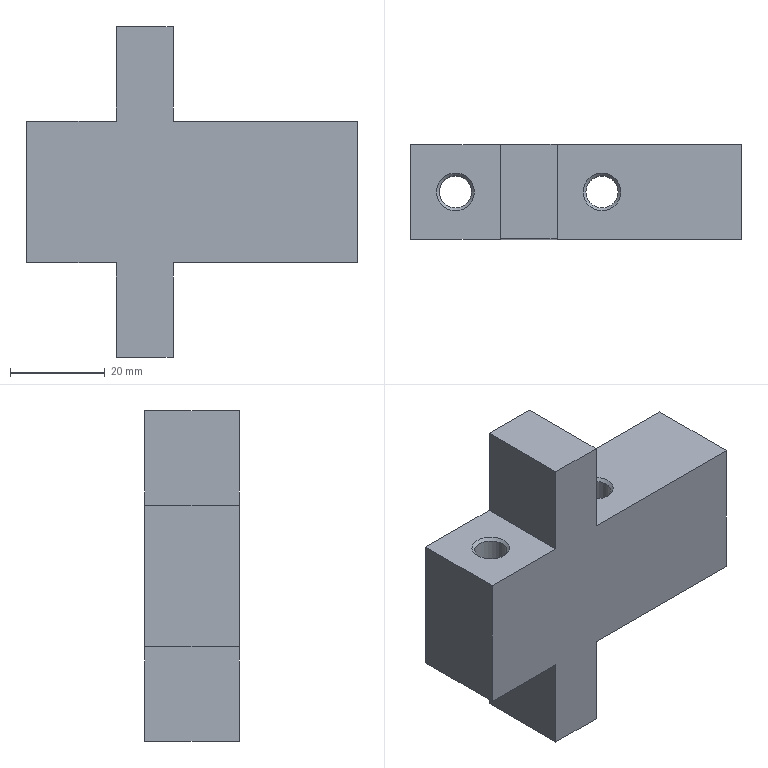Part | STEP file | 冲床-300配套压波_id182_x_t | 1 solid | 20 faces | box 70 x 20 x 70 mm | volume 49405 mm3 | plane 14 | cone 4 | cylinder 2 | commonest cylinder face diameters 6.8 x2
STEP:
#1=CARTESIAN_POINT('',(1118.5,-185.,50.));
#2=VERTEX_POINT('',#1);
#3=CARTESIAN_POINT('',(1114.5,-185.,50.));
#4=DIRECTION('',(0.,0.,-1.));
#5=DIRECTION('',(1.,0.,0.));
#6=AXIS2_PLACEMENT_3D('',#3,#4,#5);
#7=CIRCLE('',#6,4.);
#8=EDGE_CURVE('',#2,#2,#7,.T.);
#9=ORIENTED_EDGE('',*,*,#8,.T.);
#10=EDGE_LOOP('',(#9));
#11=FACE_BOUND('',#10,.T.);
#12=CARTESIAN_POINT('',(1105.,-175.,50.));
#13=VERTEX_POINT('',#12);
#14=CARTESIAN_POINT('',(1124.,-175.,50.));
#15=VERTEX_POINT('',#14);
#16=CARTESIAN_POINT('',(1155.,-175.,50.));
#17=DIRECTION('',(1.,0.,0.));
#18=VECTOR('',#17,1.);
#19=LINE('',#16,#18);
#20=EDGE_CURVE('',#13,#15,#19,.T.);
#21=ORIENTED_EDGE('',*,*,#20,.F.);
#22=CARTESIAN_POINT('',(1105.,-195.,50.));
#23=VERTEX_POINT('',#22);
#24=CARTESIAN_POINT('',(1105.,-175.,50.));
#25=DIRECTION('',(0.,1.,0.));
#26=VECTOR('',#25,1.);
#27=LINE('',#24,#26);
#28=EDGE_CURVE('',#23,#13,#27,.T.);
#29=ORIENTED_EDGE('',*,*,#28,.F.);
#30=CARTESIAN_POINT('',(1124.,-195.,50.));
#31=VERTEX_POINT('',#30);
#32=CARTESIAN_POINT('',(1155.,-195.,50.));
#33=DIRECTION('',(1.,0.,0.));
#34=VECTOR('',#33,1.);
#35=LINE('',#32,#34);
#36=EDGE_CURVE('',#23,#31,#35,.T.);
#37=ORIENTED_EDGE('',*,*,#36,.T.);
#38=CARTESIAN_POINT('',(1124.,-175.,50.));
#39=DIRECTION('',(0.,1.,0.));
#40=VECTOR('',#39,1.);
#41=LINE('',#38,#40);
#42=EDGE_CURVE('',#31,#15,#41,.T.);
#43=ORIENTED_EDGE('',*,*,#42,.T.);
#44=EDGE_LOOP('',(#21,#29,#37,#43));
#45=FACE_BOUND('',#44,.T.);
#46=CARTESIAN_POINT('',(1155.,-175.,50.));
#47=DIRECTION('',(0.,0.,1.));
#48=DIRECTION('',(-1.,0.,0.));
#49=AXIS2_PLACEMENT_3D('',#46,#47,#48);
#50=PLANE('',#49);
#51=ADVANCED_FACE('',(#11,#45),#50,.T.);
#52=CARTESIAN_POINT('',(1124.,-195.,70.));
#53=VERTEX_POINT('',#52);
#54=CARTESIAN_POINT('',(1124.,-195.,50.));
#55=DIRECTION('',(0.,0.,-1.));
#56=VECTOR('',#55,1.);
#57=LINE('',#54,#56);
#58=EDGE_CURVE('',#53,#31,#57,.T.);
#59=ORIENTED_EDGE('',*,*,#58,.F.);
#60=CARTESIAN_POINT('',(1124.,-175.,70.));
#61=VERTEX_POINT('',#60);
#62=CARTESIAN_POINT('',(1124.,-175.,70.));
#63=DIRECTION('',(0.,1.,0.));
#64=VECTOR('',#63,1.);
#65=LINE('',#62,#64);
#66=EDGE_CURVE('',#53,#61,#65,.T.);
#67=ORIENTED_EDGE('',*,*,#66,.T.);
#68=CARTESIAN_POINT('',(1124.,-175.,50.));
#69=DIRECTION('',(0.,0.,-1.));
#70=VECTOR('',#69,1.);
#71=LINE('',#68,#70);
#72=EDGE_CURVE('',#61,#15,#71,.T.);
#73=ORIENTED_EDGE('',*,*,#72,.T.);
#74=ORIENTED_EDGE('',*,*,#42,.F.);
#75=EDGE_LOOP('',(#59,#67,#73,#74));
#76=FACE_OUTER_BOUND('',#75,.T.);
#77=CARTESIAN_POINT('',(1124.,-175.,50.));
#78=DIRECTION('',(-1.,0.,0.));
#79=DIRECTION('',(0.,0.,1.));
#80=AXIS2_PLACEMENT_3D('',#77,#78,#79);
#81=PLANE('',#80);
#82=ADVANCED_FACE('',(#76),#81,.T.);
#83=CARTESIAN_POINT('',(1136.,-195.,70.));
#84=VERTEX_POINT('',#83);
#85=CARTESIAN_POINT('',(1124.,-195.,70.));
#86=DIRECTION('',(-1.,0.,0.));
#87=VECTOR('',#86,1.);
#88=LINE('',#85,#87);
#89=EDGE_CURVE('',#84,#53,#88,.T.);
#90=ORIENTED_EDGE('',*,*,#89,.F.);
#91=CARTESIAN_POINT('',(1136.,-175.,70.));
#92=VERTEX_POINT('',#91);
#93=CARTESIAN_POINT('',(1136.,-175.,70.));
#94=DIRECTION('',(0.,1.,0.));
#95=VECTOR('',#94,1.);
#96=LINE('',#93,#95);
#97=EDGE_CURVE('',#84,#92,#96,.T.);
#98=ORIENTED_EDGE('',*,*,#97,.T.);
#99=CARTESIAN_POINT('',(1124.,-175.,70.));
#100=DIRECTION('',(-1.,0.,0.));
#101=VECTOR('',#100,1.);
#102=LINE('',#99,#101);
#103=EDGE_CURVE('',#92,#61,#102,.T.);
#104=ORIENTED_EDGE('',*,*,#103,.T.);
#105=ORIENTED_EDGE('',*,*,#66,.F.);
#106=EDGE_LOOP('',(#90,#98,#104,#105));
#107=FACE_OUTER_BOUND('',#106,.T.);
#108=CARTESIAN_POINT('',(1124.,-175.,70.));
#109=DIRECTION('',(0.,0.,1.));
#110=DIRECTION('',(1.,0.,0.));
#111=AXIS2_PLACEMENT_3D('',#108,#109,#110);
#112=PLANE('',#111);
#113=ADVANCED_FACE('',(#107),#112,.T.);
#114=CARTESIAN_POINT('',(1136.,-195.,50.));
#115=VERTEX_POINT('',#114);
#116=CARTESIAN_POINT('',(1136.,-195.,70.));
#117=DIRECTION('',(0.,0.,1.));
#118=VECTOR('',#117,1.);
#119=LINE('',#116,#118);
#120=EDGE_CURVE('',#115,#84,#119,.T.);
#121=ORIENTED_EDGE('',*,*,#120,.F.);
#122=CARTESIAN_POINT('',(1136.,-175.,50.));
#123=VERTEX_POINT('',#122);
#124=CARTESIAN_POINT('',(1136.,-175.,50.));
#125=DIRECTION('',(0.,1.,0.));
#126=VECTOR('',#125,1.);
#127=LINE('',#124,#126);
#128=EDGE_CURVE('',#115,#123,#127,.T.);
#129=ORIENTED_EDGE('',*,*,#128,.T.);
#130=CARTESIAN_POINT('',(1136.,-175.,70.));
#131=DIRECTION('',(0.,0.,1.));
#132=VECTOR('',#131,1.);
#133=LINE('',#130,#132);
#134=EDGE_CURVE('',#123,#92,#133,.T.);
#135=ORIENTED_EDGE('',*,*,#134,.T.);
#136=ORIENTED_EDGE('',*,*,#97,.F.);
#137=EDGE_LOOP('',(#121,#129,#135,#136));
#138=FACE_OUTER_BOUND('',#137,.T.);
#139=CARTESIAN_POINT('',(1136.,-175.,70.));
#140=DIRECTION('',(1.,0.,0.));
#141=DIRECTION('',(0.,0.,-1.));
#142=AXIS2_PLACEMENT_3D('',#139,#140,#141);
#143=PLANE('',#142);
#144=ADVANCED_FACE('',(#138),#143,.T.);
#145=CARTESIAN_POINT('',(1149.5,-185.,50.));
#146=VERTEX_POINT('',#145);
#147=CARTESIAN_POINT('',(1145.5,-185.,50.));
#148=DIRECTION('',(0.,0.,-1.));
#149=DIRECTION('',(1.,0.,0.));
#150=AXIS2_PLACEMENT_3D('',#147,#148,#149);
#151=CIRCLE('',#150,4.);
#152=EDGE_CURVE('',#146,#146,#151,.T.);
#153=ORIENTED_EDGE('',*,*,#152,.T.);
#154=EDGE_LOOP('',(#153));
#155=FACE_BOUND('',#154,.T.);
#156=ORIENTED_EDGE('',*,*,#128,.F.);
#157=CARTESIAN_POINT('',(1175.,-195.,50.));
#158=VERTEX_POINT('',#157);
#159=CARTESIAN_POINT('',(1155.,-195.,50.));
#160=DIRECTION('',(1.,0.,0.));
#161=VECTOR('',#160,1.);
#162=LINE('',#159,#161);
#163=EDGE_CURVE('',#115,#158,#162,.T.);
#164=ORIENTED_EDGE('',*,*,#163,.T.);
#165=CARTESIAN_POINT('',(1175.,-175.,50.));
#166=VERTEX_POINT('',#165);
#167=CARTESIAN_POINT('',(1175.,-175.,50.));
#168=DIRECTION('',(0.,1.,0.));
#169=VECTOR('',#168,1.);
#170=LINE('',#167,#169);
#171=EDGE_CURVE('',#158,#166,#170,.T.);
#172=ORIENTED_EDGE('',*,*,#171,.T.);
#173=CARTESIAN_POINT('',(1155.,-175.,50.));
#174=DIRECTION('',(1.,0.,0.));
#175=VECTOR('',#174,1.);
#176=LINE('',#173,#175);
#177=EDGE_CURVE('',#123,#166,#176,.T.);
#178=ORIENTED_EDGE('',*,*,#177,.F.);
#179=EDGE_LOOP('',(#156,#164,#172,#178));
#180=FACE_BOUND('',#179,.T.);
#181=CARTESIAN_POINT('',(1155.,-175.,50.));
#182=DIRECTION('',(0.,0.,1.));
#183=DIRECTION('',(-1.,0.,0.));
#184=AXIS2_PLACEMENT_3D('',#181,#182,#183);
#185=PLANE('',#184);
#186=ADVANCED_FACE('',(#155,#180),#185,.T.);
#187=CARTESIAN_POINT('',(1175.,-175.,20.));
#188=VERTEX_POINT('',#187);
#189=CARTESIAN_POINT('',(1175.,-175.,50.));
#190=DIRECTION('',(0.,0.,1.));
#191=VECTOR('',#190,1.);
#192=LINE('',#189,#191);
#193=EDGE_CURVE('',#188,#166,#192,.T.);
#194=ORIENTED_EDGE('',*,*,#193,.T.);
#195=ORIENTED_EDGE('',*,*,#171,.F.);
#196=CARTESIAN_POINT('',(1175.,-195.,20.));
#197=VERTEX_POINT('',#196);
#198=CARTESIAN_POINT('',(1175.,-195.,50.));
#199=DIRECTION('',(0.,0.,1.));
#200=VECTOR('',#199,1.);
#201=LINE('',#198,#200);
#202=EDGE_CURVE('',#197,#158,#201,.T.);
#203=ORIENTED_EDGE('',*,*,#202,.F.);
#204=CARTESIAN_POINT('',(1175.,-175.,20.));
#205=DIRECTION('',(0.,1.,0.));
#206=VECTOR('',#205,1.);
#207=LINE('',#204,#206);
#208=EDGE_CURVE('',#197,#188,#207,.T.);
#209=ORIENTED_EDGE('',*,*,#208,.T.);
#210=EDGE_LOOP('',(#194,#195,#203,#209));
#211=FACE_OUTER_BOUND('',#210,.T.);
#212=CARTESIAN_POINT('',(1175.,-175.,50.));
#213=DIRECTION('',(-1.,0.,0.));
#214=DIRECTION('',(0.,0.,-1.));
#215=AXIS2_PLACEMENT_3D('',#212,#213,#214);
#216=PLANE('',#215);
#217=ADVANCED_FACE('',(#211),#216,.F.);
#218=CARTESIAN_POINT('',(1141.5,-185.,20.));
#219=VERTEX_POINT('',#218);
#220=CARTESIAN_POINT('',(1145.5,-185.,20.));
#221=DIRECTION('',(0.,0.,1.));
#222=DIRECTION('',(-1.,0.,0.));
#223=AXIS2_PLACEMENT_3D('',#220,#221,#222);
#224=CIRCLE('',#223,4.);
#225=EDGE_CURVE('',#219,#219,#224,.T.);
#226=ORIENTED_EDGE('',*,*,#225,.T.);
#227=EDGE_LOOP('',(#226));
#228=FACE_BOUND('',#227,.T.);
#229=CARTESIAN_POINT('',(1136.,-175.,20.));
#230=VERTEX_POINT('',#229);
#231=CARTESIAN_POINT('',(1155.,-175.,20.));
#232=DIRECTION('',(-1.,0.,0.));
#233=VECTOR('',#232,1.);
#234=LINE('',#231,#233);
#235=EDGE_CURVE('',#188,#230,#234,.T.);
#236=ORIENTED_EDGE('',*,*,#235,.F.);
#237=ORIENTED_EDGE('',*,*,#208,.F.);
#238=CARTESIAN_POINT('',(1136.,-195.,20.));
#239=VERTEX_POINT('',#238);
#240=CARTESIAN_POINT('',(1155.,-195.,20.));
#241=DIRECTION('',(-1.,0.,0.));
#242=VECTOR('',#241,1.);
#243=LINE('',#240,#242);
#244=EDGE_CURVE('',#197,#239,#243,.T.);
#245=ORIENTED_EDGE('',*,*,#244,.T.);
#246=CARTESIAN_POINT('',(1136.,-175.,20.));
#247=DIRECTION('',(0.,1.,0.));
#248=VECTOR('',#247,1.);
#249=LINE('',#246,#248);
#250=EDGE_CURVE('',#239,#230,#249,.T.);
#251=ORIENTED_EDGE('',*,*,#250,.T.);
#252=EDGE_LOOP('',(#236,#237,#245,#251));
#253=FACE_BOUND('',#252,.T.);
#254=CARTESIAN_POINT('',(1155.,-185.,20.));
#255=DIRECTION('',(0.,0.,-1.));
#256=DIRECTION('',(-1.,0.,0.));
#257=AXIS2_PLACEMENT_3D('',#254,#255,#256);
#258=PLANE('',#257);
#259=ADVANCED_FACE('',(#228,#253),#258,.T.);
#260=CARTESIAN_POINT('',(1110.5,-185.,20.));
#261=VERTEX_POINT('',#260);
#262=CARTESIAN_POINT('',(1114.5,-185.,20.));
#263=DIRECTION('',(0.,0.,1.));
#264=DIRECTION('',(-1.,0.,0.));
#265=AXIS2_PLACEMENT_3D('',#262,#263,#264);
#266=CIRCLE('',#265,4.);
#267=EDGE_CURVE('',#261,#261,#266,.T.);
#268=ORIENTED_EDGE('',*,*,#267,.T.);
#269=EDGE_LOOP('',(#268));
#270=FACE_BOUND('',#269,.T.);
#271=CARTESIAN_POINT('',(1124.,-195.,20.));
#272=VERTEX_POINT('',#271);
#273=CARTESIAN_POINT('',(1105.,-195.,20.));
#274=VERTEX_POINT('',#273);
#275=CARTESIAN_POINT('',(1155.,-195.,20.));
#276=DIRECTION('',(-1.,0.,0.));
#277=VECTOR('',#276,1.);
#278=LINE('',#275,#277);
#279=EDGE_CURVE('',#272,#274,#278,.T.);
#280=ORIENTED_EDGE('',*,*,#279,.T.);
#281=CARTESIAN_POINT('',(1105.,-175.,20.));
#282=VERTEX_POINT('',#281);
#283=CARTESIAN_POINT('',(1105.,-175.,20.));
#284=DIRECTION('',(0.,-1.,0.));
#285=VECTOR('',#284,1.);
#286=LINE('',#283,#285);
#287=EDGE_CURVE('',#282,#274,#286,.T.);
#288=ORIENTED_EDGE('',*,*,#287,.F.);
#289=CARTESIAN_POINT('',(1124.,-175.,20.));
#290=VERTEX_POINT('',#289);
#291=CARTESIAN_POINT('',(1155.,-175.,20.));
#292=DIRECTION('',(-1.,0.,0.));
#293=VECTOR('',#292,1.);
#294=LINE('',#291,#293);
#295=EDGE_CURVE('',#290,#282,#294,.T.);
#296=ORIENTED_EDGE('',*,*,#295,.F.);
#297=CARTESIAN_POINT('',(1124.,-175.,20.));
#298=DIRECTION('',(0.,-1.,0.));
#299=VECTOR('',#298,1.);
#300=LINE('',#297,#299);
#301=EDGE_CURVE('',#290,#272,#300,.T.);
#302=ORIENTED_EDGE('',*,*,#301,.T.);
#303=EDGE_LOOP('',(#280,#288,#296,#302));
#304=FACE_BOUND('',#303,.T.);
#305=CARTESIAN_POINT('',(1155.,-185.,20.));
#306=DIRECTION('',(0.,0.,-1.));
#307=DIRECTION('',(-1.,0.,0.));
#308=AXIS2_PLACEMENT_3D('',#305,#306,#307);
#309=PLANE('',#308);
#310=ADVANCED_FACE('',(#270,#304),#309,.T.);
#311=CARTESIAN_POINT('',(1105.,-195.,50.));
#312=DIRECTION('',(0.,0.,1.));
#313=VECTOR('',#312,1.);
#314=LINE('',#311,#313);
#315=EDGE_CURVE('',#274,#23,#314,.T.);
#316=ORIENTED_EDGE('',*,*,#315,.T.);
#317=ORIENTED_EDGE('',*,*,#28,.T.);
#318=CARTESIAN_POINT('',(1105.,-175.,50.));
#319=DIRECTION('',(0.,0.,1.));
#320=VECTOR('',#319,1.);
#321=LINE('',#318,#320);
#322=EDGE_CURVE('',#282,#13,#321,.T.);
#323=ORIENTED_EDGE('',*,*,#322,.F.);
#324=ORIENTED_EDGE('',*,*,#287,.T.);
#325=EDGE_LOOP('',(#316,#317,#323,#324));
#326=FACE_OUTER_BOUND('',#325,.T.);
#327=CARTESIAN_POINT('',(1105.,-175.,50.));
#328=DIRECTION('',(-1.,0.,0.));
#329=DIRECTION('',(0.,0.,-1.));
#330=AXIS2_PLACEMENT_3D('',#327,#328,#329);
#331=PLANE('',#330);
#332=ADVANCED_FACE('',(#326),#331,.T.);
#333=ORIENTED_EDGE('',*,*,#322,.T.);
#334=ORIENTED_EDGE('',*,*,#20,.T.);
#335=ORIENTED_EDGE('',*,*,#72,.F.);
#336=ORIENTED_EDGE('',*,*,#103,.F.);
#337=ORIENTED_EDGE('',*,*,#134,.F.);
#338=ORIENTED_EDGE('',*,*,#177,.T.);
#339=ORIENTED_EDGE('',*,*,#193,.F.);
#340=ORIENTED_EDGE('',*,*,#235,.T.);
#341=CARTESIAN_POINT('',(1136.,-175.,0.));
#342=VERTEX_POINT('',#341);
#343=CARTESIAN_POINT('',(1136.,-175.,0.));
#344=DIRECTION('',(0.,0.,-1.));
#345=VECTOR('',#344,1.);
#346=LINE('',#343,#345);
#347=EDGE_CURVE('',#230,#342,#346,.T.);
#348=ORIENTED_EDGE('',*,*,#347,.T.);
#349=CARTESIAN_POINT('',(1124.,-175.,0.));
#350=VERTEX_POINT('',#349);
#351=CARTESIAN_POINT('',(1124.,-175.,0.));
#352=DIRECTION('',(-1.,0.,0.));
#353=VECTOR('',#352,1.);
#354=LINE('',#351,#353);
#355=EDGE_CURVE('',#342,#350,#354,.T.);
#356=ORIENTED_EDGE('',*,*,#355,.T.);
#357=CARTESIAN_POINT('',(1124.,-175.,20.));
#358=DIRECTION('',(0.,0.,1.));
#359=VECTOR('',#358,1.);
#360=LINE('',#357,#359);
#361=EDGE_CURVE('',#350,#290,#360,.T.);
#362=ORIENTED_EDGE('',*,*,#361,.T.);
#363=ORIENTED_EDGE('',*,*,#295,.T.);
#364=EDGE_LOOP('',(#333,#334,#335,#336,#337,#338,#339,#340,#348,#356,#362,#363));
#365=FACE_OUTER_BOUND('',#364,.T.);
#366=CARTESIAN_POINT('',(1155.,-175.,50.));
#367=DIRECTION('',(0.,1.,0.));
#368=DIRECTION('',(0.,0.,-1.));
#369=AXIS2_PLACEMENT_3D('',#366,#367,#368);
#370=PLANE('',#369);
#371=ADVANCED_FACE('',(#365),#370,.T.);
#372=ORIENTED_EDGE('',*,*,#279,.F.);
#373=CARTESIAN_POINT('',(1124.,-195.,0.));
#374=VERTEX_POINT('',#373);
#375=CARTESIAN_POINT('',(1124.,-195.,20.));
#376=DIRECTION('',(0.,0.,1.));
#377=VECTOR('',#376,1.);
#378=LINE('',#375,#377);
#379=EDGE_CURVE('',#374,#272,#378,.T.);
#380=ORIENTED_EDGE('',*,*,#379,.F.);
#381=CARTESIAN_POINT('',(1136.,-195.,0.));
#382=VERTEX_POINT('',#381);
#383=CARTESIAN_POINT('',(1124.,-195.,0.));
#384=DIRECTION('',(-1.,0.,0.));
#385=VECTOR('',#384,1.);
#386=LINE('',#383,#385);
#387=EDGE_CURVE('',#382,#374,#386,.T.);
#388=ORIENTED_EDGE('',*,*,#387,.F.);
#389=CARTESIAN_POINT('',(1136.,-195.,0.));
#390=DIRECTION('',(0.,0.,-1.));
#391=VECTOR('',#390,1.);
#392=LINE('',#389,#391);
#393=EDGE_CURVE('',#239,#382,#392,.T.);
#394=ORIENTED_EDGE('',*,*,#393,.F.);
#395=ORIENTED_EDGE('',*,*,#244,.F.);
#396=ORIENTED_EDGE('',*,*,#202,.T.);
#397=ORIENTED_EDGE('',*,*,#163,.F.);
#398=ORIENTED_EDGE('',*,*,#120,.T.);
#399=ORIENTED_EDGE('',*,*,#89,.T.);
#400=ORIENTED_EDGE('',*,*,#58,.T.);
#401=ORIENTED_EDGE('',*,*,#36,.F.);
#402=ORIENTED_EDGE('',*,*,#315,.F.);
#403=EDGE_LOOP('',(#372,#380,#388,#394,#395,#396,#397,#398,#399,#400,#401,#402));
#404=FACE_OUTER_BOUND('',#403,.T.);
#405=CARTESIAN_POINT('',(1155.,-195.,50.));
#406=DIRECTION('',(0.,1.,0.));
#407=DIRECTION('',(0.,0.,-1.));
#408=AXIS2_PLACEMENT_3D('',#405,#406,#407);
#409=PLANE('',#408);
#410=ADVANCED_FACE('',(#404),#409,.F.);
#411=ORIENTED_EDGE('',*,*,#393,.T.);
#412=CARTESIAN_POINT('',(1136.,-175.,0.));
#413=DIRECTION('',(0.,-1.,0.));
#414=VECTOR('',#413,1.);
#415=LINE('',#412,#414);
#416=EDGE_CURVE('',#342,#382,#415,.T.);
#417=ORIENTED_EDGE('',*,*,#416,.F.);
#418=ORIENTED_EDGE('',*,*,#347,.F.);
#419=ORIENTED_EDGE('',*,*,#250,.F.);
#420=EDGE_LOOP('',(#411,#417,#418,#419));
#421=FACE_OUTER_BOUND('',#420,.T.);
#422=CARTESIAN_POINT('',(1136.,-175.,0.));
#423=DIRECTION('',(1.,0.,0.));
#424=DIRECTION('',(0.,0.,1.));
#425=AXIS2_PLACEMENT_3D('',#422,#423,#424);
#426=PLANE('',#425);
#427=ADVANCED_FACE('',(#421),#426,.T.);
#428=ORIENTED_EDGE('',*,*,#387,.T.);
#429=CARTESIAN_POINT('',(1124.,-175.,0.));
#430=DIRECTION('',(0.,-1.,0.));
#431=VECTOR('',#430,1.);
#432=LINE('',#429,#431);
#433=EDGE_CURVE('',#350,#374,#432,.T.);
#434=ORIENTED_EDGE('',*,*,#433,.F.);
#435=ORIENTED_EDGE('',*,*,#355,.F.);
#436=ORIENTED_EDGE('',*,*,#416,.T.);
#437=EDGE_LOOP('',(#428,#434,#435,#436));
#438=FACE_OUTER_BOUND('',#437,.T.);
#439=CARTESIAN_POINT('',(1124.,-175.,0.));
#440=DIRECTION('',(0.,0.,-1.));
#441=DIRECTION('',(1.,0.,0.));
#442=AXIS2_PLACEMENT_3D('',#439,#440,#441);
#443=PLANE('',#442);
#444=ADVANCED_FACE('',(#438),#443,.T.);
#445=ORIENTED_EDGE('',*,*,#379,.T.);
#446=ORIENTED_EDGE('',*,*,#301,.F.);
#447=ORIENTED_EDGE('',*,*,#361,.F.);
#448=ORIENTED_EDGE('',*,*,#433,.T.);
#449=EDGE_LOOP('',(#445,#446,#447,#448));
#450=FACE_OUTER_BOUND('',#449,.T.);
#451=CARTESIAN_POINT('',(1124.,-175.,20.));
#452=DIRECTION('',(-1.,0.,0.));
#453=DIRECTION('',(0.,0.,-1.));
#454=AXIS2_PLACEMENT_3D('',#451,#452,#453);
#455=PLANE('',#454);
#456=ADVANCED_FACE('',(#450),#455,.T.);
#457=CARTESIAN_POINT('',(1142.1,-185.,20.6));
#458=VERTEX_POINT('',#457);
#459=CARTESIAN_POINT('',(1145.5,-185.,20.6));
#460=DIRECTION('',(0.,0.,-1.));
#461=DIRECTION('',(-1.,0.,0.));
#462=AXIS2_PLACEMENT_3D('',#459,#460,#461);
#463=CIRCLE('',#462,3.4);
#464=EDGE_CURVE('',#458,#458,#463,.T.);
#465=ORIENTED_EDGE('',*,*,#464,.T.);
#466=EDGE_LOOP('',(#465));
#467=FACE_BOUND('',#466,.T.);
#468=CARTESIAN_POINT('',(1148.9,-185.,49.4));
#469=VERTEX_POINT('',#468);
#470=CARTESIAN_POINT('',(1145.5,-185.,49.4));
#471=DIRECTION('',(0.,0.,1.));
#472=DIRECTION('',(1.,0.,0.));
#473=AXIS2_PLACEMENT_3D('',#470,#471,#472);
#474=CIRCLE('',#473,3.4);
#475=EDGE_CURVE('',#469,#469,#474,.T.);
#476=ORIENTED_EDGE('',*,*,#475,.T.);
#477=EDGE_LOOP('',(#476));
#478=FACE_BOUND('',#477,.T.);
#479=CARTESIAN_POINT('',(1145.5,-185.,50.));
#480=DIRECTION('',(0.,0.,-1.));
#481=DIRECTION('',(-1.,0.,0.));
#482=AXIS2_PLACEMENT_3D('',#479,#480,#481);
#483=CYLINDRICAL_SURFACE('',#482,3.4);
#484=ADVANCED_FACE('',(#467,#478),#483,.F.);
#485=ORIENTED_EDGE('',*,*,#475,.F.);
#486=EDGE_LOOP('',(#485));
#487=FACE_BOUND('',#486,.T.);
#488=ORIENTED_EDGE('',*,*,#152,.F.);
#489=EDGE_LOOP('',(#488));
#490=FACE_BOUND('',#489,.T.);
#491=CARTESIAN_POINT('',(1145.5,-185.,50.));
#492=DIRECTION('',(0.,0.,1.));
#493=DIRECTION('',(1.,0.,0.));
#494=AXIS2_PLACEMENT_3D('',#491,#492,#493);
#495=CONICAL_SURFACE('',#494,4.,45.);
#496=ADVANCED_FACE('',(#487,#490),#495,.F.);
#497=ORIENTED_EDGE('',*,*,#225,.F.);
#498=EDGE_LOOP('',(#497));
#499=FACE_BOUND('',#498,.T.);
#500=ORIENTED_EDGE('',*,*,#464,.F.);
#501=EDGE_LOOP('',(#500));
#502=FACE_BOUND('',#501,.T.);
#503=CARTESIAN_POINT('',(1145.5,-185.,20.6));
#504=DIRECTION('',(0.,0.,-1.));
#505=DIRECTION('',(-1.,0.,0.));
#506=AXIS2_PLACEMENT_3D('',#503,#504,#505);
#507=CONICAL_SURFACE('',#506,3.4,45.);
#508=ADVANCED_FACE('',(#499,#502),#507,.F.);
#509=CARTESIAN_POINT('',(1111.1,-185.,20.6));
#510=VERTEX_POINT('',#509);
#511=CARTESIAN_POINT('',(1114.5,-185.,20.6));
#512=DIRECTION('',(0.,0.,-1.));
#513=DIRECTION('',(-1.,0.,0.));
#514=AXIS2_PLACEMENT_3D('',#511,#512,#513);
#515=CIRCLE('',#514,3.4);
#516=EDGE_CURVE('',#510,#510,#515,.T.);
#517=ORIENTED_EDGE('',*,*,#516,.T.);
#518=EDGE_LOOP('',(#517));
#519=FACE_BOUND('',#518,.T.);
#520=CARTESIAN_POINT('',(1117.9,-185.,49.4));
#521=VERTEX_POINT('',#520);
#522=CARTESIAN_POINT('',(1114.5,-185.,49.4));
#523=DIRECTION('',(0.,0.,1.));
#524=DIRECTION('',(1.,0.,0.));
#525=AXIS2_PLACEMENT_3D('',#522,#523,#524);
#526=CIRCLE('',#525,3.4);
#527=EDGE_CURVE('',#521,#521,#526,.T.);
#528=ORIENTED_EDGE('',*,*,#527,.T.);
#529=EDGE_LOOP('',(#528));
#530=FACE_BOUND('',#529,.T.);
#531=CARTESIAN_POINT('',(1114.5,-185.,50.));
#532=DIRECTION('',(0.,0.,-1.));
#533=DIRECTION('',(-1.,0.,0.));
#534=AXIS2_PLACEMENT_3D('',#531,#532,#533);
#535=CYLINDRICAL_SURFACE('',#534,3.4);
#536=ADVANCED_FACE('',(#519,#530),#535,.F.);
#537=ORIENTED_EDGE('',*,*,#527,.F.);
#538=EDGE_LOOP('',(#537));
#539=FACE_BOUND('',#538,.T.);
#540=ORIENTED_EDGE('',*,*,#8,.F.);
#541=EDGE_LOOP('',(#540));
#542=FACE_BOUND('',#541,.T.);
#543=CARTESIAN_POINT('',(1114.5,-185.,50.));
#544=DIRECTION('',(0.,0.,1.));
#545=DIRECTION('',(1.,0.,0.));
#546=AXIS2_PLACEMENT_3D('',#543,#544,#545);
#547=CONICAL_SURFACE('',#546,4.,45.);
#548=ADVANCED_FACE('',(#539,#542),#547,.F.);
#549=ORIENTED_EDGE('',*,*,#267,.F.);
#550=EDGE_LOOP('',(#549));
#551=FACE_BOUND('',#550,.T.);
#552=ORIENTED_EDGE('',*,*,#516,.F.);
#553=EDGE_LOOP('',(#552));
#554=FACE_BOUND('',#553,.T.);
#555=CARTESIAN_POINT('',(1114.5,-185.,20.6));
#556=DIRECTION('',(0.,0.,-1.));
#557=DIRECTION('',(-1.,0.,0.));
#558=AXIS2_PLACEMENT_3D('',#555,#556,#557);
#559=CONICAL_SURFACE('',#558,3.4,45.);
#560=ADVANCED_FACE('',(#551,#554),#559,.F.);
#561=CLOSED_SHELL('',(#51,#82,#113,#144,#186,#217,#259,#310,#332,#371,#410,#427,#444,#456,#484,#496,#508,#536,#548,#560));
#562=MANIFOLD_SOLID_BREP('',#561);
#563=(LENGTH_UNIT()NAMED_UNIT(*)SI_UNIT(.MILLI.,.METRE.));
#564=UNCERTAINTY_MEASURE_WITH_UNIT(LENGTH_MEASURE(0.00002),#563,'','');
#565=(NAMED_UNIT(*)PLANE_ANGLE_UNIT()SI_UNIT($,.RADIAN.));
#566=PLANE_ANGLE_MEASURE_WITH_UNIT(PLANE_ANGLE_MEASURE(0.01745),#565);
#567=DIMENSIONAL_EXPONENTS(0.,0.,0.,0.,0.,0.,0.);
#568=(CONVERSION_BASED_UNIT('DEGREE',#566)NAMED_UNIT(#567)PLANE_ANGLE_UNIT());
#569=(NAMED_UNIT(*)SI_UNIT($,.STERADIAN.)SOLID_ANGLE_UNIT());
#570=(GEOMETRIC_REPRESENTATION_CONTEXT(3)GLOBAL_UNCERTAINTY_ASSIGNED_CONTEXT((#564))GLOBAL_UNIT_ASSIGNED_CONTEXT((#563,#568,#569))REPRESENTATION_CONTEXT('',''));
#571=ADVANCED_BREP_SHAPE_REPRESENTATION('',(#562),#570);